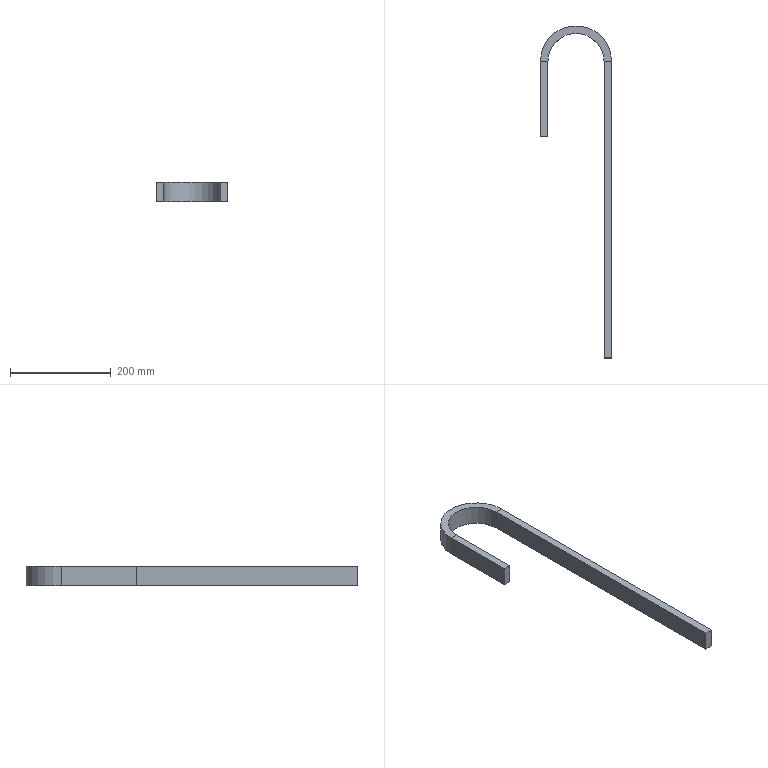Part | SolidWorks | features BaseBody 1 | 1 solid | 14 faces | box 141.75 x 660.875 x 38.9 mm | volume 551169 mm3 | plane 12 | cylinder 2 | commonest cylinder face diameters 111.57 x1 141.75 x1
STEP:
#1=CARTESIAN_POINT('',(119.115,-440.,-19.45));
#2=VERTEX_POINT('',#1);
#3=CARTESIAN_POINT('',(134.205,-440.,-19.45));
#4=VERTEX_POINT('',#3);
#5=CARTESIAN_POINT('',(134.205,-440.,-19.45));
#6=DIRECTION('',(1.,0.,0.));
#7=VECTOR('',#6,1000.);
#8=LINE('',#5,#7);
#9=EDGE_CURVE('',#2,#4,#8,.T.);
#10=ORIENTED_EDGE('',*,*,#9,.F.);
#11=CARTESIAN_POINT('',(119.115,150.,-19.45));
#12=VERTEX_POINT('',#11);
#13=CARTESIAN_POINT('',(119.115,150.,-19.45));
#14=DIRECTION('',(0.,-1.,0.));
#15=VECTOR('',#14,1000.);
#16=LINE('',#13,#15);
#17=EDGE_CURVE('',#12,#2,#16,.T.);
#18=ORIENTED_EDGE('',*,*,#17,.F.);
#19=CARTESIAN_POINT('',(134.205,150.,-19.45));
#20=VERTEX_POINT('',#19);
#21=CARTESIAN_POINT('',(134.205,150.,-19.45));
#22=DIRECTION('',(1.,0.,0.));
#23=VECTOR('',#22,1000.);
#24=LINE('',#21,#23);
#25=EDGE_CURVE('',#12,#20,#24,.T.);
#26=ORIENTED_EDGE('',*,*,#25,.T.);
#27=CARTESIAN_POINT('',(134.205,150.,-19.45));
#28=DIRECTION('',(0.,-1.,0.));
#29=VECTOR('',#28,1000.);
#30=LINE('',#27,#29);
#31=EDGE_CURVE('',#20,#4,#30,.T.);
#32=ORIENTED_EDGE('',*,*,#31,.T.);
#33=EDGE_LOOP('',(#10,#18,#26,#32));
#34=FACE_OUTER_BOUND('',#33,.T.);
#35=CARTESIAN_POINT('',(134.205,150.,-19.45));
#36=DIRECTION('',(0.,0.,-1.));
#37=DIRECTION('',(-1.,0.,0.));
#38=AXIS2_PLACEMENT_3D('',#35,#36,#37);
#39=PLANE('',#38);
#40=ADVANCED_FACE('',(#34),#39,.T.);
#41=ORIENTED_EDGE('',*,*,#17,.T.);
#42=CARTESIAN_POINT('',(119.115,-440.,19.45));
#43=VERTEX_POINT('',#42);
#44=CARTESIAN_POINT('',(119.115,-440.,-19.45));
#45=DIRECTION('',(0.,0.,-1.));
#46=VECTOR('',#45,1000.);
#47=LINE('',#44,#46);
#48=EDGE_CURVE('',#43,#2,#47,.T.);
#49=ORIENTED_EDGE('',*,*,#48,.F.);
#50=CARTESIAN_POINT('',(119.115,150.,19.45));
#51=VERTEX_POINT('',#50);
#52=CARTESIAN_POINT('',(119.115,150.,19.45));
#53=DIRECTION('',(0.,-1.,0.));
#54=VECTOR('',#53,1000.);
#55=LINE('',#52,#54);
#56=EDGE_CURVE('',#51,#43,#55,.T.);
#57=ORIENTED_EDGE('',*,*,#56,.F.);
#58=CARTESIAN_POINT('',(119.115,150.,-19.45));
#59=DIRECTION('',(0.,0.,-1.));
#60=VECTOR('',#59,1000.);
#61=LINE('',#58,#60);
#62=EDGE_CURVE('',#51,#12,#61,.T.);
#63=ORIENTED_EDGE('',*,*,#62,.T.);
#64=EDGE_LOOP('',(#41,#49,#57,#63));
#65=FACE_OUTER_BOUND('',#64,.T.);
#66=CARTESIAN_POINT('',(119.115,150.,-19.45));
#67=DIRECTION('',(-1.,0.,0.));
#68=DIRECTION('',(0.,-1.,0.));
#69=AXIS2_PLACEMENT_3D('',#66,#67,#68);
#70=PLANE('',#69);
#71=ADVANCED_FACE('',(#65),#70,.T.);
#72=ORIENTED_EDGE('',*,*,#56,.T.);
#73=CARTESIAN_POINT('',(134.205,-440.,19.45));
#74=VERTEX_POINT('',#73);
#75=CARTESIAN_POINT('',(134.205,-440.,19.45));
#76=DIRECTION('',(-1.,0.,0.));
#77=VECTOR('',#76,1000.);
#78=LINE('',#75,#77);
#79=EDGE_CURVE('',#74,#43,#78,.T.);
#80=ORIENTED_EDGE('',*,*,#79,.F.);
#81=CARTESIAN_POINT('',(134.205,150.,19.45));
#82=VERTEX_POINT('',#81);
#83=CARTESIAN_POINT('',(134.205,150.,19.45));
#84=DIRECTION('',(0.,-1.,0.));
#85=VECTOR('',#84,1000.);
#86=LINE('',#83,#85);
#87=EDGE_CURVE('',#82,#74,#86,.T.);
#88=ORIENTED_EDGE('',*,*,#87,.F.);
#89=CARTESIAN_POINT('',(134.205,150.,19.45));
#90=DIRECTION('',(-1.,0.,0.));
#91=VECTOR('',#90,1000.);
#92=LINE('',#89,#91);
#93=EDGE_CURVE('',#82,#51,#92,.T.);
#94=ORIENTED_EDGE('',*,*,#93,.T.);
#95=EDGE_LOOP('',(#72,#80,#88,#94));
#96=FACE_OUTER_BOUND('',#95,.T.);
#97=CARTESIAN_POINT('',(134.205,150.,19.45));
#98=DIRECTION('',(0.,0.,1.));
#99=DIRECTION('',(1.,0.,0.));
#100=AXIS2_PLACEMENT_3D('',#97,#98,#99);
#101=PLANE('',#100);
#102=ADVANCED_FACE('',(#96),#101,.T.);
#103=ORIENTED_EDGE('',*,*,#87,.T.);
#104=CARTESIAN_POINT('',(134.205,-440.,-19.45));
#105=DIRECTION('',(0.,0.,1.));
#106=VECTOR('',#105,1000.);
#107=LINE('',#104,#106);
#108=EDGE_CURVE('',#4,#74,#107,.T.);
#109=ORIENTED_EDGE('',*,*,#108,.F.);
#110=ORIENTED_EDGE('',*,*,#31,.F.);
#111=CARTESIAN_POINT('',(134.205,150.,-19.45));
#112=DIRECTION('',(0.,0.,1.));
#113=VECTOR('',#112,1000.);
#114=LINE('',#111,#113);
#115=EDGE_CURVE('',#20,#82,#114,.T.);
#116=ORIENTED_EDGE('',*,*,#115,.T.);
#117=EDGE_LOOP('',(#103,#109,#110,#116));
#118=FACE_OUTER_BOUND('',#117,.T.);
#119=CARTESIAN_POINT('',(134.205,150.,-19.45));
#120=DIRECTION('',(1.,0.,0.));
#121=DIRECTION('',(0.,1.,0.));
#122=AXIS2_PLACEMENT_3D('',#119,#120,#121);
#123=PLANE('',#122);
#124=ADVANCED_FACE('',(#118),#123,.T.);
#125=ORIENTED_EDGE('',*,*,#25,.F.);
#126=CARTESIAN_POINT('',(7.545,150.,-19.45));
#127=VERTEX_POINT('',#126);
#128=CARTESIAN_POINT('',(63.33,150.,-19.45));
#129=DIRECTION('',(0.,0.,-1.));
#130=DIRECTION('',(-1.,0.,0.));
#131=AXIS2_PLACEMENT_3D('',#128,#129,#130);
#132=CIRCLE('',#131,55.785);
#133=EDGE_CURVE('',#127,#12,#132,.T.);
#134=ORIENTED_EDGE('',*,*,#133,.F.);
#135=CARTESIAN_POINT('',(-7.545,150.,-19.45));
#136=VERTEX_POINT('',#135);
#137=CARTESIAN_POINT('',(-7.545,150.,-19.45));
#138=DIRECTION('',(-1.,0.,0.));
#139=VECTOR('',#138,1000.);
#140=LINE('',#137,#139);
#141=EDGE_CURVE('',#127,#136,#140,.T.);
#142=ORIENTED_EDGE('',*,*,#141,.T.);
#143=CARTESIAN_POINT('',(63.33,150.,-19.45));
#144=DIRECTION('',(0.,0.,-1.));
#145=DIRECTION('',(-1.,0.,0.));
#146=AXIS2_PLACEMENT_3D('',#143,#144,#145);
#147=CIRCLE('',#146,70.875);
#148=EDGE_CURVE('',#136,#20,#147,.T.);
#149=ORIENTED_EDGE('',*,*,#148,.T.);
#150=EDGE_LOOP('',(#125,#134,#142,#149));
#151=FACE_OUTER_BOUND('',#150,.T.);
#152=CARTESIAN_POINT('',(-7.545,150.,-19.45));
#153=DIRECTION('',(0.,0.,-1.));
#154=DIRECTION('',(-1.,0.,0.));
#155=AXIS2_PLACEMENT_3D('',#152,#153,#154);
#156=PLANE('',#155);
#157=ADVANCED_FACE('',(#151),#156,.T.);
#158=ORIENTED_EDGE('',*,*,#133,.T.);
#159=ORIENTED_EDGE('',*,*,#62,.F.);
#160=CARTESIAN_POINT('',(7.545,150.,19.45));
#161=VERTEX_POINT('',#160);
#162=CARTESIAN_POINT('',(63.33,150.,19.45));
#163=DIRECTION('',(0.,0.,-1.));
#164=DIRECTION('',(-1.,0.,0.));
#165=AXIS2_PLACEMENT_3D('',#162,#163,#164);
#166=CIRCLE('',#165,55.785);
#167=EDGE_CURVE('',#161,#51,#166,.T.);
#168=ORIENTED_EDGE('',*,*,#167,.F.);
#169=CARTESIAN_POINT('',(7.545,150.,-19.45));
#170=DIRECTION('',(0.,0.,-1.));
#171=VECTOR('',#170,1000.);
#172=LINE('',#169,#171);
#173=EDGE_CURVE('',#161,#127,#172,.T.);
#174=ORIENTED_EDGE('',*,*,#173,.T.);
#175=EDGE_LOOP('',(#158,#159,#168,#174));
#176=FACE_OUTER_BOUND('',#175,.T.);
#177=CARTESIAN_POINT('',(63.33,150.,0.));
#178=DIRECTION('',(0.,0.,-1.));
#179=DIRECTION('',(-1.,0.,0.));
#180=AXIS2_PLACEMENT_3D('',#177,#178,#179);
#181=CYLINDRICAL_SURFACE('',#180,55.785);
#182=ADVANCED_FACE('',(#176),#181,.F.);
#183=ORIENTED_EDGE('',*,*,#167,.T.);
#184=ORIENTED_EDGE('',*,*,#93,.F.);
#185=CARTESIAN_POINT('',(-7.545,150.,19.45));
#186=VERTEX_POINT('',#185);
#187=CARTESIAN_POINT('',(63.33,150.,19.45));
#188=DIRECTION('',(0.,0.,-1.));
#189=DIRECTION('',(-1.,0.,0.));
#190=AXIS2_PLACEMENT_3D('',#187,#188,#189);
#191=CIRCLE('',#190,70.875);
#192=EDGE_CURVE('',#186,#82,#191,.T.);
#193=ORIENTED_EDGE('',*,*,#192,.F.);
#194=CARTESIAN_POINT('',(-7.545,150.,19.45));
#195=DIRECTION('',(1.,0.,0.));
#196=VECTOR('',#195,1000.);
#197=LINE('',#194,#196);
#198=EDGE_CURVE('',#186,#161,#197,.T.);
#199=ORIENTED_EDGE('',*,*,#198,.T.);
#200=EDGE_LOOP('',(#183,#184,#193,#199));
#201=FACE_OUTER_BOUND('',#200,.T.);
#202=CARTESIAN_POINT('',(-7.545,150.,19.45));
#203=DIRECTION('',(0.,0.,1.));
#204=DIRECTION('',(1.,0.,0.));
#205=AXIS2_PLACEMENT_3D('',#202,#203,#204);
#206=PLANE('',#205);
#207=ADVANCED_FACE('',(#201),#206,.T.);
#208=ORIENTED_EDGE('',*,*,#192,.T.);
#209=ORIENTED_EDGE('',*,*,#115,.F.);
#210=ORIENTED_EDGE('',*,*,#148,.F.);
#211=CARTESIAN_POINT('',(-7.545,150.,-19.45));
#212=DIRECTION('',(0.,0.,1.));
#213=VECTOR('',#212,1000.);
#214=LINE('',#211,#213);
#215=EDGE_CURVE('',#136,#186,#214,.T.);
#216=ORIENTED_EDGE('',*,*,#215,.T.);
#217=EDGE_LOOP('',(#208,#209,#210,#216));
#218=FACE_OUTER_BOUND('',#217,.T.);
#219=CARTESIAN_POINT('',(63.33,150.,0.));
#220=DIRECTION('',(0.,0.,-1.));
#221=DIRECTION('',(-1.,0.,0.));
#222=AXIS2_PLACEMENT_3D('',#219,#220,#221);
#223=CYLINDRICAL_SURFACE('',#222,70.875);
#224=ADVANCED_FACE('',(#218),#223,.T.);
#225=ORIENTED_EDGE('',*,*,#141,.F.);
#226=CARTESIAN_POINT('',(7.545,0.,-19.45));
#227=VERTEX_POINT('',#226);
#228=CARTESIAN_POINT('',(7.545,0.,-19.45));
#229=DIRECTION('',(0.,1.,0.));
#230=VECTOR('',#229,1000.);
#231=LINE('',#228,#230);
#232=EDGE_CURVE('',#227,#127,#231,.T.);
#233=ORIENTED_EDGE('',*,*,#232,.F.);
#234=CARTESIAN_POINT('',(-7.545,0.,-19.45));
#235=VERTEX_POINT('',#234);
#236=CARTESIAN_POINT('',(-7.545,0.,-19.45));
#237=DIRECTION('',(-1.,0.,0.));
#238=VECTOR('',#237,1000.);
#239=LINE('',#236,#238);
#240=EDGE_CURVE('',#227,#235,#239,.T.);
#241=ORIENTED_EDGE('',*,*,#240,.T.);
#242=CARTESIAN_POINT('',(-7.545,0.,-19.45));
#243=DIRECTION('',(0.,1.,0.));
#244=VECTOR('',#243,1000.);
#245=LINE('',#242,#244);
#246=EDGE_CURVE('',#235,#136,#245,.T.);
#247=ORIENTED_EDGE('',*,*,#246,.T.);
#248=EDGE_LOOP('',(#225,#233,#241,#247));
#249=FACE_OUTER_BOUND('',#248,.T.);
#250=CARTESIAN_POINT('',(-7.545,0.,-19.45));
#251=DIRECTION('',(0.,0.,-1.));
#252=DIRECTION('',(-1.,0.,0.));
#253=AXIS2_PLACEMENT_3D('',#250,#251,#252);
#254=PLANE('',#253);
#255=ADVANCED_FACE('',(#249),#254,.T.);
#256=ORIENTED_EDGE('',*,*,#232,.T.);
#257=ORIENTED_EDGE('',*,*,#173,.F.);
#258=CARTESIAN_POINT('',(7.545,0.,19.45));
#259=VERTEX_POINT('',#258);
#260=CARTESIAN_POINT('',(7.545,0.,19.45));
#261=DIRECTION('',(0.,1.,0.));
#262=VECTOR('',#261,1000.);
#263=LINE('',#260,#262);
#264=EDGE_CURVE('',#259,#161,#263,.T.);
#265=ORIENTED_EDGE('',*,*,#264,.F.);
#266=CARTESIAN_POINT('',(7.545,0.,-19.45));
#267=DIRECTION('',(0.,0.,-1.));
#268=VECTOR('',#267,1000.);
#269=LINE('',#266,#268);
#270=EDGE_CURVE('',#259,#227,#269,.T.);
#271=ORIENTED_EDGE('',*,*,#270,.T.);
#272=EDGE_LOOP('',(#256,#257,#265,#271));
#273=FACE_OUTER_BOUND('',#272,.T.);
#274=CARTESIAN_POINT('',(7.545,0.,-19.45));
#275=DIRECTION('',(1.,0.,0.));
#276=DIRECTION('',(0.,0.,-1.));
#277=AXIS2_PLACEMENT_3D('',#274,#275,#276);
#278=PLANE('',#277);
#279=ADVANCED_FACE('',(#273),#278,.T.);
#280=ORIENTED_EDGE('',*,*,#264,.T.);
#281=ORIENTED_EDGE('',*,*,#198,.F.);
#282=CARTESIAN_POINT('',(-7.545,0.,19.45));
#283=VERTEX_POINT('',#282);
#284=CARTESIAN_POINT('',(-7.545,0.,19.45));
#285=DIRECTION('',(0.,1.,0.));
#286=VECTOR('',#285,1000.);
#287=LINE('',#284,#286);
#288=EDGE_CURVE('',#283,#186,#287,.T.);
#289=ORIENTED_EDGE('',*,*,#288,.F.);
#290=CARTESIAN_POINT('',(-7.545,0.,19.45));
#291=DIRECTION('',(1.,0.,0.));
#292=VECTOR('',#291,1000.);
#293=LINE('',#290,#292);
#294=EDGE_CURVE('',#283,#259,#293,.T.);
#295=ORIENTED_EDGE('',*,*,#294,.T.);
#296=EDGE_LOOP('',(#280,#281,#289,#295));
#297=FACE_OUTER_BOUND('',#296,.T.);
#298=CARTESIAN_POINT('',(-7.545,0.,19.45));
#299=DIRECTION('',(0.,0.,1.));
#300=DIRECTION('',(1.,0.,0.));
#301=AXIS2_PLACEMENT_3D('',#298,#299,#300);
#302=PLANE('',#301);
#303=ADVANCED_FACE('',(#297),#302,.T.);
#304=ORIENTED_EDGE('',*,*,#288,.T.);
#305=ORIENTED_EDGE('',*,*,#215,.F.);
#306=ORIENTED_EDGE('',*,*,#246,.F.);
#307=CARTESIAN_POINT('',(-7.545,0.,-19.45));
#308=DIRECTION('',(0.,0.,1.));
#309=VECTOR('',#308,1000.);
#310=LINE('',#307,#309);
#311=EDGE_CURVE('',#235,#283,#310,.T.);
#312=ORIENTED_EDGE('',*,*,#311,.T.);
#313=EDGE_LOOP('',(#304,#305,#306,#312));
#314=FACE_OUTER_BOUND('',#313,.T.);
#315=CARTESIAN_POINT('',(-7.545,0.,-19.45));
#316=DIRECTION('',(-1.,0.,0.));
#317=DIRECTION('',(0.,0.,1.));
#318=AXIS2_PLACEMENT_3D('',#315,#316,#317);
#319=PLANE('',#318);
#320=ADVANCED_FACE('',(#314),#319,.T.);
#321=ORIENTED_EDGE('',*,*,#48,.T.);
#322=ORIENTED_EDGE('',*,*,#9,.T.);
#323=ORIENTED_EDGE('',*,*,#108,.T.);
#324=ORIENTED_EDGE('',*,*,#79,.T.);
#325=EDGE_LOOP('',(#321,#322,#323,#324));
#326=FACE_OUTER_BOUND('',#325,.T.);
#327=CARTESIAN_POINT('',(126.66,-440.,0.));
#328=DIRECTION('',(0.,-1.,0.));
#329=DIRECTION('',(0.,0.,1.));
#330=AXIS2_PLACEMENT_3D('',#327,#328,#329);
#331=PLANE('',#330);
#332=ADVANCED_FACE('',(#326),#331,.T.);
#333=ORIENTED_EDGE('',*,*,#270,.F.);
#334=ORIENTED_EDGE('',*,*,#294,.F.);
#335=ORIENTED_EDGE('',*,*,#311,.F.);
#336=ORIENTED_EDGE('',*,*,#240,.F.);
#337=EDGE_LOOP('',(#333,#334,#335,#336));
#338=FACE_OUTER_BOUND('',#337,.T.);
#339=CARTESIAN_POINT('',(0.,0.,0.));
#340=DIRECTION('',(0.,1.,0.));
#341=DIRECTION('',(0.,0.,1.));
#342=AXIS2_PLACEMENT_3D('',#339,#340,#341);
#343=PLANE('',#342);
#344=ADVANCED_FACE('',(#338),#343,.F.);
#345=CLOSED_SHELL('',(#40,#71,#102,#124,#157,#182,#207,#224,#255,#279,#303,#320,#332,#344));
#346=MANIFOLD_SOLID_BREP('',#345);
#347=CARTESIAN_POINT('',(0.,0.,0.));
#348=DIRECTION('',(0.,0.,1.));
#349=DIRECTION('',(1.,0.,0.));
#350=AXIS2_PLACEMENT_3D('',#347,#348,#349);
#351=(LENGTH_UNIT()NAMED_UNIT(*)SI_UNIT(.MILLI.,.METRE.));
#352=UNCERTAINTY_MEASURE_WITH_UNIT(LENGTH_MEASURE(0.00001),#351,'','');
#353=(NAMED_UNIT(*)PLANE_ANGLE_UNIT()SI_UNIT($,.RADIAN.));
#354=(NAMED_UNIT(*)SI_UNIT($,.STERADIAN.)SOLID_ANGLE_UNIT());
#355=(GEOMETRIC_REPRESENTATION_CONTEXT(3)GLOBAL_UNCERTAINTY_ASSIGNED_CONTEXT((#352))GLOBAL_UNIT_ASSIGNED_CONTEXT((#351,#353,#354))REPRESENTATION_CONTEXT('',''));
#356=ADVANCED_BREP_SHAPE_REPRESENTATION('',(#346,#350),#355);